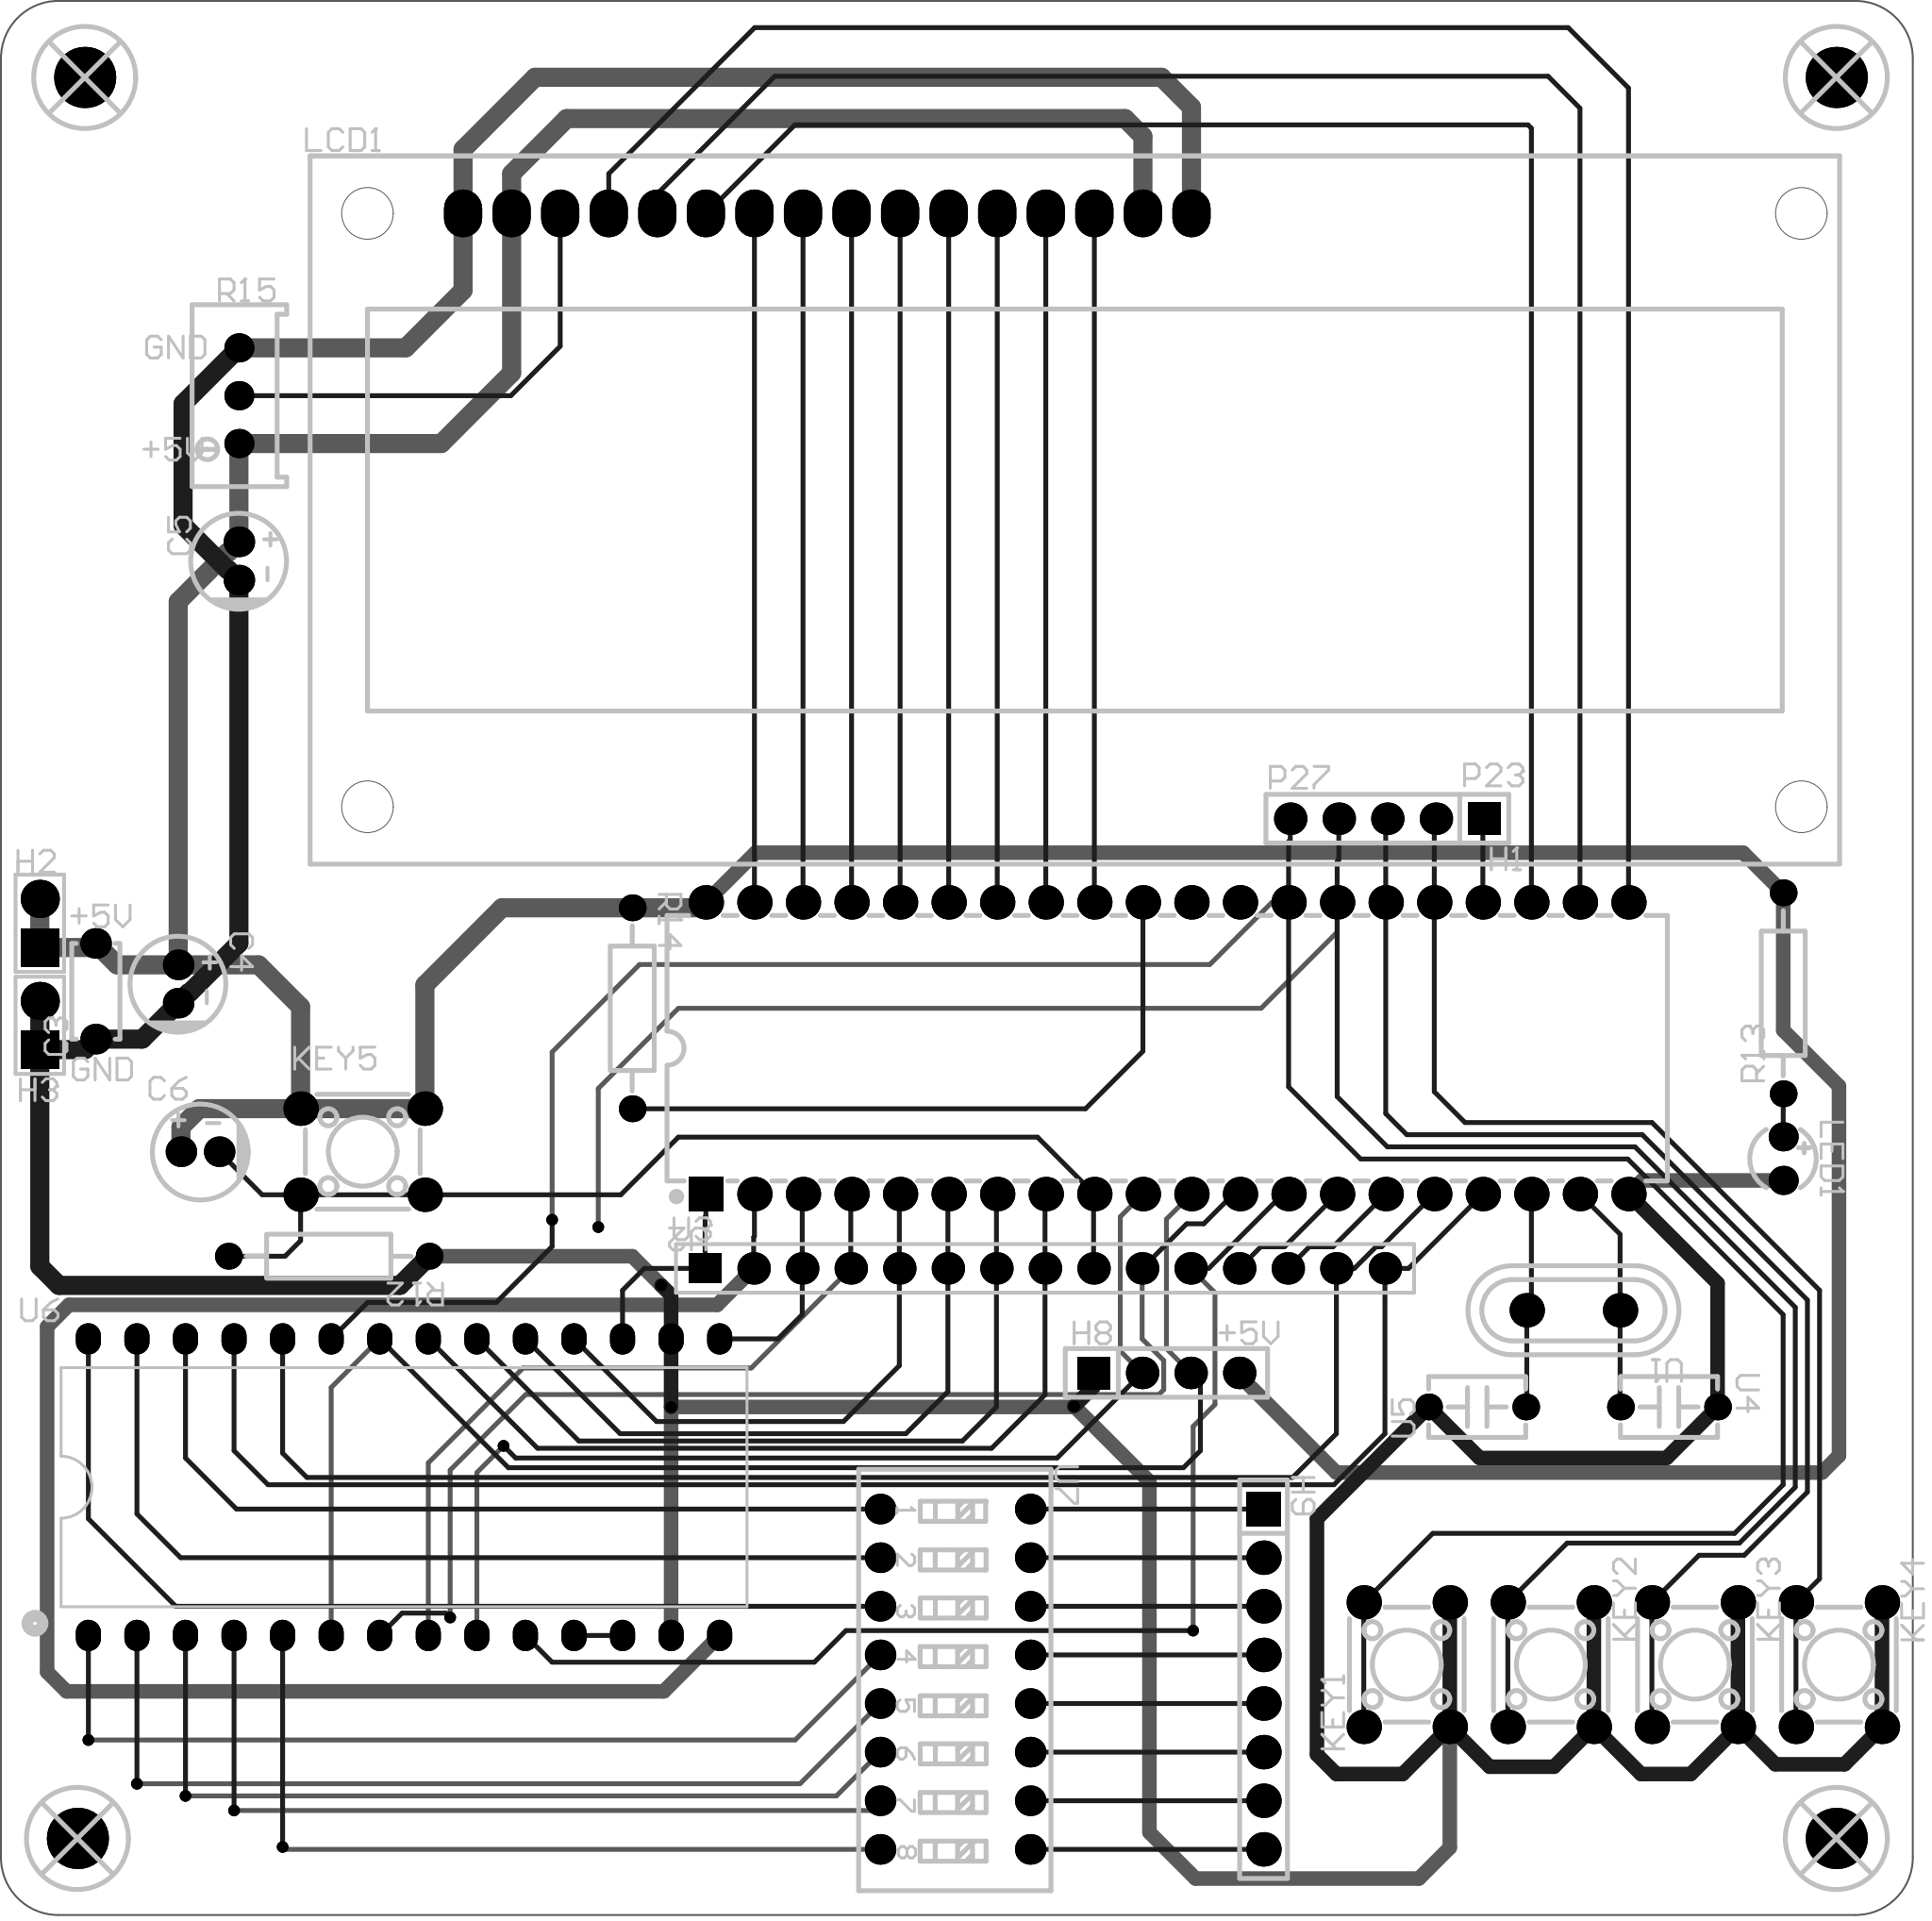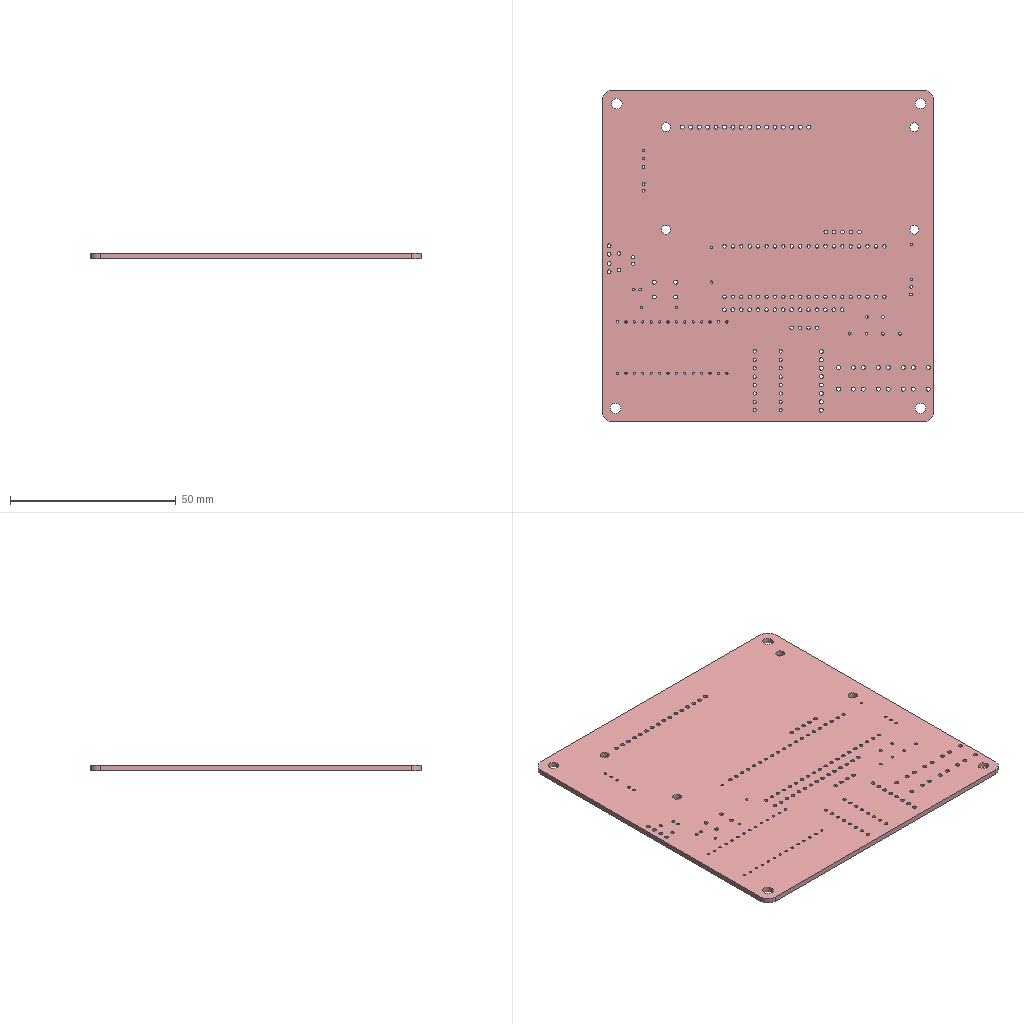Circuit board layout | Altium Designer | box 100 x 100 x 1.6 mm
Layer stack:
# Altium Designer layer stack of  (unit mm; dielectric type: 0 none, 1 core, 2 prepreg, 3 surface material)
index,name,kind,layer,copper_thickness_mm,dielectric_type,dielectric_thickness_mm,dielectric_material,dielectric_constant
0,Top Paste Mask Layer,other,,,,,,
1,Top Silkscreen Layer,other,,,,,,
2,Top Solder Mask Layer,dielectric,,,3,0.01,,3.3
3,Top Layer,copper,Top Layer,0.035,,,,
4,Dielectric1,dielectric,,,3,1.51,FR4,4.5
5,Bottom Layer,copper,Bottom Layer,0.035,,,,
6,Bottom Solder Mask Layer,dielectric,,,3,0.01,,3.3
7,Bottom Silkscreen Layer,other,,,,,,
8,Bottom Paste Mask Layer,other,,,,,,
# drill layer pairs: low layer,high layer
drill_pair,Top Layer,Bottom Layer
Part placement:
Designator,Comment,Layer,Footprint,Center-X(mm),Center-Y(mm),Rotation
SCREW1,,TopLayer,M3螺丝,80.2,80.2,0
C3,100nF,TopLayer,CAP-TH_L5.0-W2.5-P5.00-D1.0,81.153,124.46,90
SCREW2,,TopLayer,M3螺丝,172.2,80.2,0
SCREW3,,TopLayer,M3螺丝,80.581,172.2,0
SCREW4,,TopLayer,M3螺丝,172.2,172.2,0
C4,10uF,TopLayer,CAP-TH_BD5.0-P2.00-D0.5-FD-A,85.471,124.841,270
C5,10uF,TopLayer,CAP-TH_BD5.0-P2.00-D0.5-FD-A,88.646,146.939,270
C6,10uF,TopLayer,CAP-TH_BD5.0-P2.00-D0.5-FD-A,86.614,116.078,0
H1,PZ254V-11-05P,TopLayer,HDR-TH_5P-P2.54-V-M,148.717,133.477,180
H2,PZ254V-11-02P,TopLayer,HDR-TH_2P-P2.54-V-M,78.232,128.016,90
H3,PZ254V-11-02P,TopLayer,HDR-TH_2P-P2.54-V-M,78.232,122.682,90
LCD1,LCM1602K-NSW-BBW,TopLayer,MODULE-TH_LCM1602K,119.421,165.1,0
LED1,3A2RUD,TopLayer,LED-TH_BD3.5-P2.28_3A2RUC,169.423,115.718,270
U2,STC89C516RD+40I-PDIP40,TopLayer,DIP-40_L52.3-W13.9-P2.54-LS15.2-BL,137.201,121.485,0
U3,ZX-PM2.54-1-15PY,TopLayer,HDR-TH_15P-P2.54-V-F,130.81,109.982,0
U1,12MHz,TopLayer,HC-49S_L11.0-W4.7-P4.88,158.45,107.795,180
H8,,TopLayer,HDR-TH_4P-P2.54-V-F,137.16,104.521,0
KEY1,,TopLayer,SW-TH_4P-L6.0-W6.0-P4.50-LS6.5,149.733,89.281,270
KEY2,,TopLayer,SW-TH_4P-L6.0-W6.0-P4.50-LS6.5,157.268,89.281,270
KEY3,,TopLayer,SW-TH_4P-L6.0-W6.0-P4.50-LS6.5,164.804,89.281,270
KEY4,,TopLayer,SW-TH_4P-L6.0-W6.0-P4.50-LS6.5,172.339,89.281,270
R12,10kΩ,TopLayer,RES-TH_BD2.3-L6.5-P10.50-D0.5,93.345,110.617,180
R13,10kΩ,TopLayer,RES-TH_BD2.3-L6.5-P10.50-D0.5,169.423,124.354,90
R14,10kΩ,TopLayer,RES-TH_BD2.3-L6.5-P10.50-D0.5,109.22,123.571,270
U4,33pF,TopLayer,CAP-TH_L5.0-W2.5-P5.08-D0.7,163.449,102.743,180
U5,33pF,TopLayer,CAP-TH_L5.0-W2.5-P5.08-D0.7,153.416,102.743,0
KEY5,,TopLayer,SW-TH_4P-L6.0-W6.0-P4.50-LS6.5,95.123,116.078,180
R15,10kΩ,TopLayer,RES-ADJ-TH_3P-L10.0-W10.0-P2.50-L,88.646,155.575,90
H9,,TopLayer,HDR-TH_8P-P2.54-V-F-1,142.24,88.519,270
U6,ADC0809-N,TopLayer,PDIP-28_L36.0-W13.0-P2.54-LS15.5-BL,97.282,98.552,0
U7,2.54插件8位拨码开关,TopLayer,SW-TH_16P-L21.9-W9.9-P2.54-LS7.8,126.111,88.519,270
Pad and via stacks:
# Altium Designer via and pad stacks of  (unit mm). Each distinct definition once, with the count of objects using it.
# via: kind,start_layer,end_layer,hole_mm,diameter_mm,mode(0 simple;1 top-mid-bottom;2 full stack),diameter_per_layer,count,example_net
# pad: kind,layer,hole_mm,hole_type(0 round;1 square;2 slot),plating,top_size,top_shape(1 round;2 rect;3 octagon;9 rounded rect),mid_size,bottom_size,mode,footprint,size_per_layer,count,example
pad,Multi-Layer,3.2,0,plated,3.2x3.2,1,3.2x3.2,3.2x3.2,0,M3\u00C2\u00DD\u00CB\u00BF,,4,SCREW1.1
pad,Multi-Layer,1,0,plated,1.6x1.6,1,1.6x1.6,1.6x1.6,0,CAP-TH_L5.0-W2.5-P5.00-D1.0,,2,C3.1
pad,Multi-Layer,0.9,0,plated,1.6x1.6,1,1.6x1.6,1.6x1.6,0,CAP-TH_BD5.0-P2.00-D0.5-FD-A,,6,C4.2
pad,Multi-Layer,1.1,0,plated,1.7x1.7,2,1.7x1.7,1.7x1.7,0,HDR-TH_5P-P2.54-V-M,,1,H1.1
pad,Multi-Layer,1.1,0,plated,1.7x1.7,1,1.7x1.7,1.7x1.7,0,HDR-TH_5P-P2.54-V-M,,4,H1.2
pad,Multi-Layer,1.2,0,plated,2x2,2,2x2,2x2,0,HDR-TH_2P-P2.54-V-M,,2,H2.1
pad,Multi-Layer,1.2,0,plated,2x2,1,2x2,2x2,0,HDR-TH_2P-P2.54-V-M,,2,H2.2
pad,Multi-Layer,1.2,0,plated,2.5x2,1,2.5x2,2.5x2,0,MODULE-TH_LCM1602K,,16,LCD1.1
pad,Multi-Layer,0.9144,0,plated,1.524x1.524,1,1.524x1.524,1.524x1.524,0,LED-TH_BD3.5-P2.28_3A2RUC,,2,LED1.2
pad,Multi-Layer,1,0,plated,1.8x1.8,1,1.8x1.8,1.8x1.8,0,DIP-40_L52.3-W13.9-P2.54-LS15.2-BL,,39,U2.19
pad,Multi-Layer,1,0,plated,1.8x1.8,2,1.8x1.8,1.8x1.8,0,DIP-40_L52.3-W13.9-P2.54-LS15.2-BL,,1,U2.1
pad,Multi-Layer,1.1,0,plated,1.7x1.7,1,1.7x1.7,1.7x1.7,0,HDR-TH_15P-P2.54-V-F,,14,U3.15
pad,Multi-Layer,1.1,0,plated,1.7x1.575,2,1.7x1.575,1.7x1.575,0,HDR-TH_15P-P2.54-V-F,,1,U3.1
pad,Multi-Layer,0.9,0,plated,1.8x1.8,1,1.8x1.8,1.8x1.8,0,HC-49S_L11.0-W4.7-P4.88,,2,U1.1
pad,Multi-Layer,1.1,0,plated,1.7x1.7,2,1.7x1.7,1.7x1.7,0,HDR-TH_4P-P2.54-V-F,,1,H8.1
pad,Multi-Layer,1.1,0,plated,1.7x1.7,1,1.7x1.7,1.7x1.7,0,HDR-TH_4P-P2.54-V-F,,3,H8.2
pad,Multi-Layer,1.2,0,plated,1.8x1.8,1,1.8x1.8,1.8x1.8,0,SW-TH_4P-L6.0-W6.0-P4.50-LS6.5,,20,KEY1.1
pad,Multi-Layer,0.7,0,plated,1.4x1.4,1,1.4x1.4,1.4x1.4,0,RES-TH_BD2.3-L6.5-P10.50-D0.5,,6,R12.1
pad,Multi-Layer,0.8,0,plated,1.4x1.4,1,1.4x1.4,1.4x1.4,0,CAP-TH_L5.0-W2.5-P5.08-D0.7,,4,U4.1
pad,Multi-Layer,0.762,0,plated,1.524x1.524,1,1.524x1.524,1.524x1.524,0,RES-ADJ-TH_3P-L10.0-W10.0-P2.50-L,,3,R15.2
pad,Multi-Layer,1.2,0,plated,1.8x1.8,2,1.8x1.8,1.8x1.8,0,HDR-TH_8P-P2.54-V-F-1,,1,H9.1
pad,Multi-Layer,1.2,0,plated,1.8x1.8,1,1.8x1.8,1.8x1.8,0,HDR-TH_8P-P2.54-V-F-1,,7,H9.2
pad,Multi-Layer,0.7,0,plated,1.314x1.643,1,1.314x1.643,1.314x1.643,0,PDIP-28_L36.0-W13.0-P2.54-LS15.5-BL,,28,U6.1
pad,Multi-Layer,1,0,plated,1.6x1.6,1,1.6x1.6,1.6x1.6,0,SW-TH_16P-L21.9-W9.9-P2.54-LS7.8,,16,U7.9
via,Top Layer,Bottom Layer,0.3048,0.61,0,,13,P27